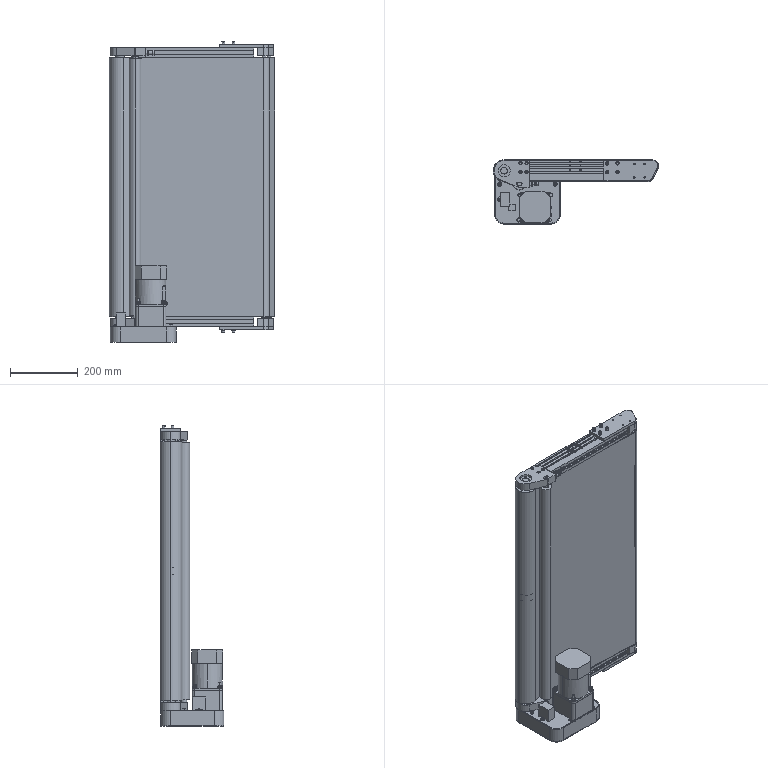Part | SolidWorks | 16 solids | 2274 faces | box 489 x 188.5 x 889 mm | volume 10301612 mm3 | plane 1429 | cylinder 585 | cone 174 | spline 68 | torus 16 | sphere 2 | commonest cylinder face diameters 5 x132 8.5 x60 10 x54 12 x37 9.2 x28 6 x24